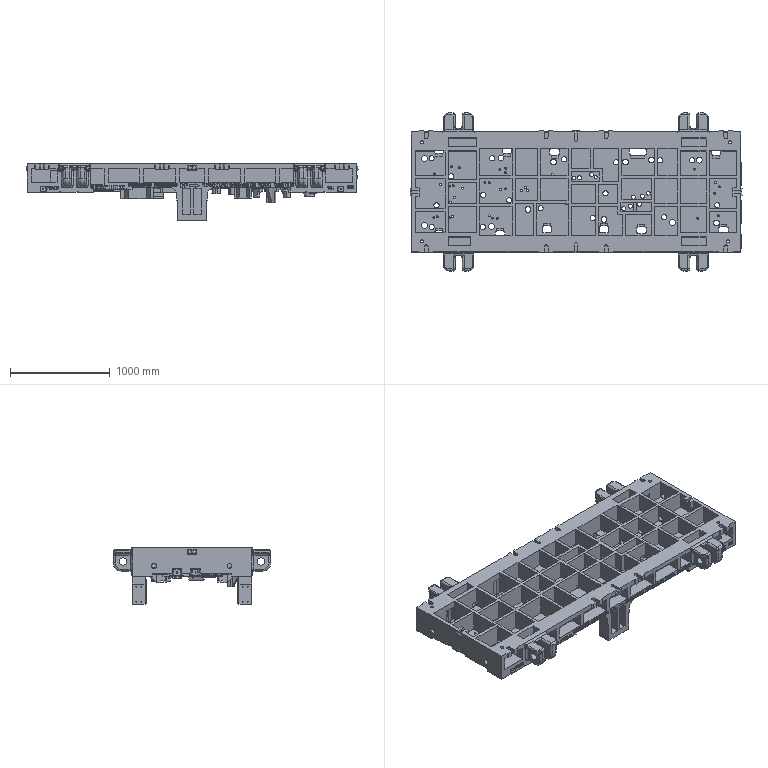Part | STEP file | gslz 2016.10.28-13_id6_x_t | 1 solid | 5791 faces | volume 504665580 mm3 | plane 3390 | cylinder 993 | other 773 | cone 450 | torus 88 | spline 81 | sphere 16 | commonest cylinder face diameters 40 x142 10.3 x133 6.8 x125 20 x106 5.2 x89 8.5 x54